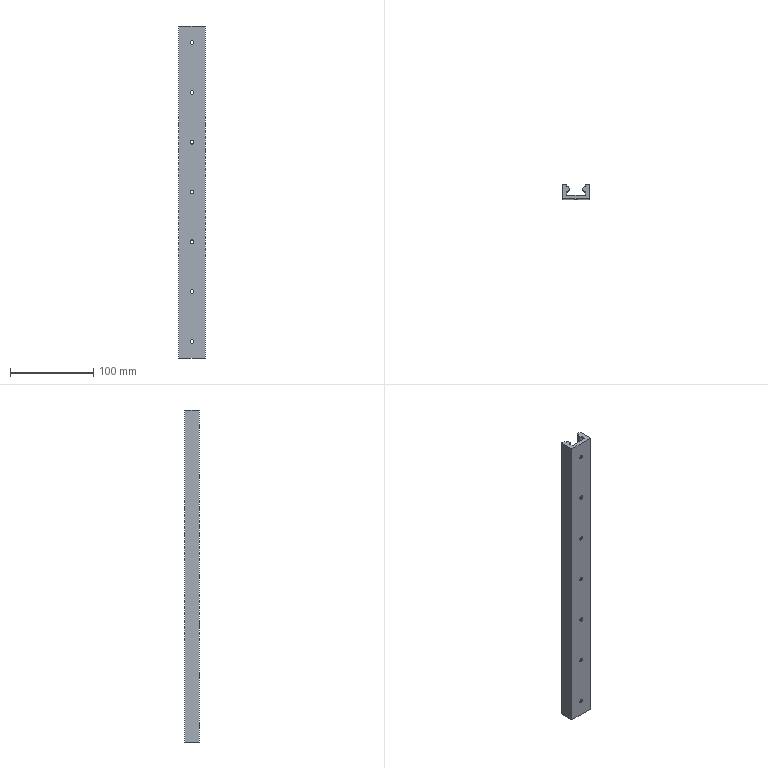Part | SolidWorks | features BaseBody 1 | 1 solid | 50 faces | box 32 x 17.5 x 400 mm | volume 119366 mm3 | cylinder 31 | plane 19 | commonest cylinder face diameters 4.5 x14 8 x14 6 x3
STEP:
#1=CARTESIAN_POINT('',(-16.,0.,400.));
#2=VERTEX_POINT('',#1);
#3=CARTESIAN_POINT('',(-10.95,0.,400.));
#4=VERTEX_POINT('',#3);
#5=CARTESIAN_POINT('',(-16.,0.,400.));
#6=DIRECTION('',(1.,0.,0.));
#7=VECTOR('',#6,1000.);
#8=LINE('',#5,#7);
#9=EDGE_CURVE('',#2,#4,#8,.T.);
#10=ORIENTED_EDGE('',*,*,#9,.F.);
#11=CARTESIAN_POINT('',(-16.,-17.5,400.));
#12=VERTEX_POINT('',#11);
#13=CARTESIAN_POINT('',(-16.,600.853,400.));
#14=DIRECTION('',(0.,-1.,0.));
#15=VECTOR('',#14,1000.);
#16=LINE('',#13,#15);
#17=EDGE_CURVE('',#2,#12,#16,.T.);
#18=ORIENTED_EDGE('',*,*,#17,.T.);
#19=CARTESIAN_POINT('',(16.,-17.5,400.));
#20=VERTEX_POINT('',#19);
#21=CARTESIAN_POINT('',(-16.,-17.5,400.));
#22=DIRECTION('',(1.,0.,0.));
#23=VECTOR('',#22,1000.);
#24=LINE('',#21,#23);
#25=EDGE_CURVE('',#12,#20,#24,.T.);
#26=ORIENTED_EDGE('',*,*,#25,.T.);
#27=CARTESIAN_POINT('',(16.,0.,400.));
#28=VERTEX_POINT('',#27);
#29=CARTESIAN_POINT('',(16.,600.853,400.));
#30=DIRECTION('',(0.,-1.,0.));
#31=VECTOR('',#30,1000.);
#32=LINE('',#29,#31);
#33=EDGE_CURVE('',#28,#20,#32,.T.);
#34=ORIENTED_EDGE('',*,*,#33,.F.);
#35=CARTESIAN_POINT('',(10.95,0.,400.));
#36=VERTEX_POINT('',#35);
#37=CARTESIAN_POINT('',(-16.,0.,400.));
#38=DIRECTION('',(1.,0.,0.));
#39=VECTOR('',#38,1000.);
#40=LINE('',#37,#39);
#41=EDGE_CURVE('',#36,#28,#40,.T.);
#42=ORIENTED_EDGE('',*,*,#41,.F.);
#43=CARTESIAN_POINT('',(10.95,-2.7,400.));
#44=VERTEX_POINT('',#43);
#45=CARTESIAN_POINT('',(10.95,0.,400.));
#46=DIRECTION('',(0.,1.,0.));
#47=VECTOR('',#46,1000.);
#48=LINE('',#45,#47);
#49=EDGE_CURVE('',#44,#36,#48,.T.);
#50=ORIENTED_EDGE('',*,*,#49,.F.);
#51=CARTESIAN_POINT('',(7.95,-5.7,400.));
#52=VERTEX_POINT('',#51);
#53=CARTESIAN_POINT('',(10.95,-5.7,400.));
#54=DIRECTION('',(0.,0.,1.));
#55=DIRECTION('',(-1.,0.,0.));
#56=AXIS2_PLACEMENT_3D('',#53,#54,#55);
#57=CIRCLE('',#56,3.);
#58=EDGE_CURVE('',#44,#52,#57,.T.);
#59=ORIENTED_EDGE('',*,*,#58,.T.);
#60=CARTESIAN_POINT('',(10.95,-8.7,400.));
#61=VERTEX_POINT('',#60);
#62=CARTESIAN_POINT('',(10.95,-5.7,400.));
#63=DIRECTION('',(0.,0.,1.));
#64=DIRECTION('',(-1.,0.,0.));
#65=AXIS2_PLACEMENT_3D('',#62,#63,#64);
#66=CIRCLE('',#65,3.);
#67=EDGE_CURVE('',#52,#61,#66,.T.);
#68=ORIENTED_EDGE('',*,*,#67,.T.);
#69=CARTESIAN_POINT('',(10.95,-13.1,400.));
#70=VERTEX_POINT('',#69);
#71=CARTESIAN_POINT('',(10.95,-8.7,400.));
#72=DIRECTION('',(0.,1.,0.));
#73=VECTOR('',#72,1000.);
#74=LINE('',#71,#73);
#75=EDGE_CURVE('',#70,#61,#74,.T.);
#76=ORIENTED_EDGE('',*,*,#75,.F.);
#77=CARTESIAN_POINT('',(-10.95,-13.1,400.));
#78=VERTEX_POINT('',#77);
#79=CARTESIAN_POINT('',(10.95,-13.1,400.));
#80=DIRECTION('',(1.,0.,0.));
#81=VECTOR('',#80,1000.);
#82=LINE('',#79,#81);
#83=EDGE_CURVE('',#78,#70,#82,.T.);
#84=ORIENTED_EDGE('',*,*,#83,.F.);
#85=CARTESIAN_POINT('',(-10.95,-8.7,400.));
#86=VERTEX_POINT('',#85);
#87=CARTESIAN_POINT('',(-10.95,-13.1,400.));
#88=DIRECTION('',(0.,-1.,0.));
#89=VECTOR('',#88,1000.);
#90=LINE('',#87,#89);
#91=EDGE_CURVE('',#86,#78,#90,.T.);
#92=ORIENTED_EDGE('',*,*,#91,.F.);
#93=CARTESIAN_POINT('',(-10.95,-2.7,400.));
#94=VERTEX_POINT('',#93);
#95=CARTESIAN_POINT('',(-10.95,-5.7,400.));
#96=DIRECTION('',(0.,0.,1.));
#97=DIRECTION('',(-1.,0.,0.));
#98=AXIS2_PLACEMENT_3D('',#95,#96,#97);
#99=CIRCLE('',#98,3.);
#100=EDGE_CURVE('',#86,#94,#99,.T.);
#101=ORIENTED_EDGE('',*,*,#100,.T.);
#102=CARTESIAN_POINT('',(-10.95,-2.7,400.));
#103=DIRECTION('',(0.,-1.,0.));
#104=VECTOR('',#103,1000.);
#105=LINE('',#102,#104);
#106=EDGE_CURVE('',#4,#94,#105,.T.);
#107=ORIENTED_EDGE('',*,*,#106,.F.);
#108=EDGE_LOOP('',(#10,#18,#26,#34,#42,#50,#59,#68,#76,#84,#92,#101,#107));
#109=FACE_OUTER_BOUND('',#108,.T.);
#110=CARTESIAN_POINT('',(-16.,600.853,400.));
#111=DIRECTION('',(0.,0.,-1.));
#112=DIRECTION('',(0.,-1.,0.));
#113=AXIS2_PLACEMENT_3D('',#110,#111,#112);
#114=PLANE('',#113);
#115=ADVANCED_FACE('',(#109),#114,.F.);
#116=CARTESIAN_POINT('',(0.,-16.,76.));
#117=VERTEX_POINT('',#116);
#118=CARTESIAN_POINT('',(0.,-16.,84.));
#119=VERTEX_POINT('',#118);
#120=CARTESIAN_POINT('',(0.,-16.,80.));
#121=DIRECTION('',(0.,1.,0.));
#122=DIRECTION('',(0.,0.,1.));
#123=AXIS2_PLACEMENT_3D('',#120,#121,#122);
#124=CIRCLE('',#123,4.);
#125=EDGE_CURVE('',#117,#119,#124,.T.);
#126=ORIENTED_EDGE('',*,*,#125,.F.);
#127=CARTESIAN_POINT('',(0.,-13.1,76.));
#128=VERTEX_POINT('',#127);
#129=CARTESIAN_POINT('',(0.,-13.1,76.));
#130=DIRECTION('',(0.,1.,0.));
#131=VECTOR('',#130,1000.);
#132=LINE('',#129,#131);
#133=EDGE_CURVE('',#117,#128,#132,.T.);
#134=ORIENTED_EDGE('',*,*,#133,.T.);
#135=CARTESIAN_POINT('',(0.,-13.1,84.));
#136=VERTEX_POINT('',#135);
#137=CARTESIAN_POINT('',(0.,-13.1,80.));
#138=DIRECTION('',(0.,1.,0.));
#139=DIRECTION('',(0.,0.,1.));
#140=AXIS2_PLACEMENT_3D('',#137,#138,#139);
#141=CIRCLE('',#140,4.);
#142=EDGE_CURVE('',#128,#136,#141,.T.);
#143=ORIENTED_EDGE('',*,*,#142,.T.);
#144=CARTESIAN_POINT('',(0.,-13.1,84.));
#145=DIRECTION('',(0.,1.,0.));
#146=VECTOR('',#145,1000.);
#147=LINE('',#144,#146);
#148=EDGE_CURVE('',#119,#136,#147,.T.);
#149=ORIENTED_EDGE('',*,*,#148,.F.);
#150=EDGE_LOOP('',(#126,#134,#143,#149));
#151=FACE_OUTER_BOUND('',#150,.T.);
#152=CARTESIAN_POINT('',(0.,-13.1,80.));
#153=DIRECTION('',(0.,1.,0.));
#154=DIRECTION('',(0.,0.,1.));
#155=AXIS2_PLACEMENT_3D('',#152,#153,#154);
#156=CYLINDRICAL_SURFACE('',#155,4.);
#157=ADVANCED_FACE('',(#151),#156,.F.);
#158=CARTESIAN_POINT('',(0.,-17.5,77.75));
#159=VERTEX_POINT('',#158);
#160=CARTESIAN_POINT('',(0.,-17.5,82.25));
#161=VERTEX_POINT('',#160);
#162=CARTESIAN_POINT('',(0.,-17.5,80.));
#163=DIRECTION('',(0.,1.,0.));
#164=DIRECTION('',(0.,0.,1.));
#165=AXIS2_PLACEMENT_3D('',#162,#163,#164);
#166=CIRCLE('',#165,2.25);
#167=EDGE_CURVE('',#159,#161,#166,.T.);
#168=ORIENTED_EDGE('',*,*,#167,.F.);
#169=CARTESIAN_POINT('',(0.,-16.,77.75));
#170=VERTEX_POINT('',#169);
#171=CARTESIAN_POINT('',(0.,-13.1,77.75));
#172=DIRECTION('',(0.,1.,0.));
#173=VECTOR('',#172,1000.);
#174=LINE('',#171,#173);
#175=EDGE_CURVE('',#159,#170,#174,.T.);
#176=ORIENTED_EDGE('',*,*,#175,.T.);
#177=CARTESIAN_POINT('',(0.,-16.,82.25));
#178=VERTEX_POINT('',#177);
#179=CARTESIAN_POINT('',(0.,-16.,80.));
#180=DIRECTION('',(0.,1.,0.));
#181=DIRECTION('',(0.,0.,1.));
#182=AXIS2_PLACEMENT_3D('',#179,#180,#181);
#183=CIRCLE('',#182,2.25);
#184=EDGE_CURVE('',#170,#178,#183,.T.);
#185=ORIENTED_EDGE('',*,*,#184,.T.);
#186=CARTESIAN_POINT('',(0.,-13.1,82.25));
#187=DIRECTION('',(0.,1.,0.));
#188=VECTOR('',#187,1000.);
#189=LINE('',#186,#188);
#190=EDGE_CURVE('',#161,#178,#189,.T.);
#191=ORIENTED_EDGE('',*,*,#190,.F.);
#192=EDGE_LOOP('',(#168,#176,#185,#191));
#193=FACE_OUTER_BOUND('',#192,.T.);
#194=CARTESIAN_POINT('',(0.,-13.1,80.));
#195=DIRECTION('',(0.,1.,0.));
#196=DIRECTION('',(0.,0.,1.));
#197=AXIS2_PLACEMENT_3D('',#194,#195,#196);
#198=CYLINDRICAL_SURFACE('',#197,2.25);
#199=ADVANCED_FACE('',(#193),#198,.F.);
#200=CARTESIAN_POINT('',(0.,-16.,16.));
#201=VERTEX_POINT('',#200);
#202=CARTESIAN_POINT('',(0.,-16.,24.));
#203=VERTEX_POINT('',#202);
#204=CARTESIAN_POINT('',(0.,-16.,20.));
#205=DIRECTION('',(0.,1.,0.));
#206=DIRECTION('',(0.,0.,1.));
#207=AXIS2_PLACEMENT_3D('',#204,#205,#206);
#208=CIRCLE('',#207,4.);
#209=EDGE_CURVE('',#201,#203,#208,.T.);
#210=ORIENTED_EDGE('',*,*,#209,.F.);
#211=CARTESIAN_POINT('',(0.,-13.1,16.));
#212=VERTEX_POINT('',#211);
#213=CARTESIAN_POINT('',(0.,-13.1,16.));
#214=DIRECTION('',(0.,1.,0.));
#215=VECTOR('',#214,1000.);
#216=LINE('',#213,#215);
#217=EDGE_CURVE('',#201,#212,#216,.T.);
#218=ORIENTED_EDGE('',*,*,#217,.T.);
#219=CARTESIAN_POINT('',(0.,-13.1,24.));
#220=VERTEX_POINT('',#219);
#221=CARTESIAN_POINT('',(0.,-13.1,20.));
#222=DIRECTION('',(0.,1.,0.));
#223=DIRECTION('',(0.,0.,1.));
#224=AXIS2_PLACEMENT_3D('',#221,#222,#223);
#225=CIRCLE('',#224,4.);
#226=EDGE_CURVE('',#212,#220,#225,.T.);
#227=ORIENTED_EDGE('',*,*,#226,.T.);
#228=CARTESIAN_POINT('',(0.,-13.1,24.));
#229=DIRECTION('',(0.,1.,0.));
#230=VECTOR('',#229,1000.);
#231=LINE('',#228,#230);
#232=EDGE_CURVE('',#203,#220,#231,.T.);
#233=ORIENTED_EDGE('',*,*,#232,.F.);
#234=EDGE_LOOP('',(#210,#218,#227,#233));
#235=FACE_OUTER_BOUND('',#234,.T.);
#236=CARTESIAN_POINT('',(0.,-13.1,20.));
#237=DIRECTION('',(0.,1.,0.));
#238=DIRECTION('',(0.,0.,1.));
#239=AXIS2_PLACEMENT_3D('',#236,#237,#238);
#240=CYLINDRICAL_SURFACE('',#239,4.);
#241=ADVANCED_FACE('',(#235),#240,.F.);
#242=CARTESIAN_POINT('',(0.,-17.5,17.75));
#243=VERTEX_POINT('',#242);
#244=CARTESIAN_POINT('',(0.,-17.5,22.25));
#245=VERTEX_POINT('',#244);
#246=CARTESIAN_POINT('',(0.,-17.5,20.));
#247=DIRECTION('',(0.,1.,0.));
#248=DIRECTION('',(0.,0.,1.));
#249=AXIS2_PLACEMENT_3D('',#246,#247,#248);
#250=CIRCLE('',#249,2.25);
#251=EDGE_CURVE('',#243,#245,#250,.T.);
#252=ORIENTED_EDGE('',*,*,#251,.F.);
#253=CARTESIAN_POINT('',(0.,-16.,17.75));
#254=VERTEX_POINT('',#253);
#255=CARTESIAN_POINT('',(0.,-13.1,17.75));
#256=DIRECTION('',(0.,1.,0.));
#257=VECTOR('',#256,1000.);
#258=LINE('',#255,#257);
#259=EDGE_CURVE('',#243,#254,#258,.T.);
#260=ORIENTED_EDGE('',*,*,#259,.T.);
#261=CARTESIAN_POINT('',(0.,-16.,22.25));
#262=VERTEX_POINT('',#261);
#263=CARTESIAN_POINT('',(0.,-16.,20.));
#264=DIRECTION('',(0.,1.,0.));
#265=DIRECTION('',(0.,0.,1.));
#266=AXIS2_PLACEMENT_3D('',#263,#264,#265);
#267=CIRCLE('',#266,2.25);
#268=EDGE_CURVE('',#254,#262,#267,.T.);
#269=ORIENTED_EDGE('',*,*,#268,.T.);
#270=CARTESIAN_POINT('',(0.,-13.1,22.25));
#271=DIRECTION('',(0.,1.,0.));
#272=VECTOR('',#271,1000.);
#273=LINE('',#270,#272);
#274=EDGE_CURVE('',#245,#262,#273,.T.);
#275=ORIENTED_EDGE('',*,*,#274,.F.);
#276=EDGE_LOOP('',(#252,#260,#269,#275));
#277=FACE_OUTER_BOUND('',#276,.T.);
#278=CARTESIAN_POINT('',(0.,-13.1,20.));
#279=DIRECTION('',(0.,1.,0.));
#280=DIRECTION('',(0.,0.,1.));
#281=AXIS2_PLACEMENT_3D('',#278,#279,#280);
#282=CYLINDRICAL_SURFACE('',#281,2.25);
#283=ADVANCED_FACE('',(#277),#282,.F.);
#284=CARTESIAN_POINT('',(0.,-16.,136.));
#285=VERTEX_POINT('',#284);
#286=CARTESIAN_POINT('',(0.,-16.,144.));
#287=VERTEX_POINT('',#286);
#288=CARTESIAN_POINT('',(0.,-16.,140.));
#289=DIRECTION('',(0.,1.,0.));
#290=DIRECTION('',(0.,0.,1.));
#291=AXIS2_PLACEMENT_3D('',#288,#289,#290);
#292=CIRCLE('',#291,4.);
#293=EDGE_CURVE('',#285,#287,#292,.T.);
#294=ORIENTED_EDGE('',*,*,#293,.F.);
#295=CARTESIAN_POINT('',(0.,-13.1,136.));
#296=VERTEX_POINT('',#295);
#297=CARTESIAN_POINT('',(0.,-13.1,136.));
#298=DIRECTION('',(0.,1.,0.));
#299=VECTOR('',#298,1000.);
#300=LINE('',#297,#299);
#301=EDGE_CURVE('',#285,#296,#300,.T.);
#302=ORIENTED_EDGE('',*,*,#301,.T.);
#303=CARTESIAN_POINT('',(0.,-13.1,144.));
#304=VERTEX_POINT('',#303);
#305=CARTESIAN_POINT('',(0.,-13.1,140.));
#306=DIRECTION('',(0.,1.,0.));
#307=DIRECTION('',(0.,0.,1.));
#308=AXIS2_PLACEMENT_3D('',#305,#306,#307);
#309=CIRCLE('',#308,4.);
#310=EDGE_CURVE('',#296,#304,#309,.T.);
#311=ORIENTED_EDGE('',*,*,#310,.T.);
#312=CARTESIAN_POINT('',(0.,-13.1,144.));
#313=DIRECTION('',(0.,1.,0.));
#314=VECTOR('',#313,1000.);
#315=LINE('',#312,#314);
#316=EDGE_CURVE('',#287,#304,#315,.T.);
#317=ORIENTED_EDGE('',*,*,#316,.F.);
#318=EDGE_LOOP('',(#294,#302,#311,#317));
#319=FACE_OUTER_BOUND('',#318,.T.);
#320=CARTESIAN_POINT('',(0.,-13.1,140.));
#321=DIRECTION('',(0.,1.,0.));
#322=DIRECTION('',(0.,0.,1.));
#323=AXIS2_PLACEMENT_3D('',#320,#321,#322);
#324=CYLINDRICAL_SURFACE('',#323,4.);
#325=ADVANCED_FACE('',(#319),#324,.F.);
#326=CARTESIAN_POINT('',(0.,-17.5,137.75));
#327=VERTEX_POINT('',#326);
#328=CARTESIAN_POINT('',(0.,-17.5,142.25));
#329=VERTEX_POINT('',#328);
#330=CARTESIAN_POINT('',(0.,-17.5,140.));
#331=DIRECTION('',(0.,1.,0.));
#332=DIRECTION('',(0.,0.,1.));
#333=AXIS2_PLACEMENT_3D('',#330,#331,#332);
#334=CIRCLE('',#333,2.25);
#335=EDGE_CURVE('',#327,#329,#334,.T.);
#336=ORIENTED_EDGE('',*,*,#335,.F.);
#337=CARTESIAN_POINT('',(0.,-16.,137.75));
#338=VERTEX_POINT('',#337);
#339=CARTESIAN_POINT('',(0.,-13.1,137.75));
#340=DIRECTION('',(0.,1.,0.));
#341=VECTOR('',#340,1000.);
#342=LINE('',#339,#341);
#343=EDGE_CURVE('',#327,#338,#342,.T.);
#344=ORIENTED_EDGE('',*,*,#343,.T.);
#345=CARTESIAN_POINT('',(0.,-16.,142.25));
#346=VERTEX_POINT('',#345);
#347=CARTESIAN_POINT('',(0.,-16.,140.));
#348=DIRECTION('',(0.,1.,0.));
#349=DIRECTION('',(0.,0.,1.));
#350=AXIS2_PLACEMENT_3D('',#347,#348,#349);
#351=CIRCLE('',#350,2.25);
#352=EDGE_CURVE('',#338,#346,#351,.T.);
#353=ORIENTED_EDGE('',*,*,#352,.T.);
#354=CARTESIAN_POINT('',(0.,-13.1,142.25));
#355=DIRECTION('',(0.,1.,0.));
#356=VECTOR('',#355,1000.);
#357=LINE('',#354,#356);
#358=EDGE_CURVE('',#329,#346,#357,.T.);
#359=ORIENTED_EDGE('',*,*,#358,.F.);
#360=EDGE_LOOP('',(#336,#344,#353,#359));
#361=FACE_OUTER_BOUND('',#360,.T.);
#362=CARTESIAN_POINT('',(0.,-13.1,140.));
#363=DIRECTION('',(0.,1.,0.));
#364=DIRECTION('',(0.,0.,1.));
#365=AXIS2_PLACEMENT_3D('',#362,#363,#364);
#366=CYLINDRICAL_SURFACE('',#365,2.25);
#367=ADVANCED_FACE('',(#361),#366,.F.);
#368=CARTESIAN_POINT('',(0.,-16.,196.));
#369=VERTEX_POINT('',#368);
#370=CARTESIAN_POINT('',(0.,-16.,204.));
#371=VERTEX_POINT('',#370);
#372=CARTESIAN_POINT('',(0.,-16.,200.));
#373=DIRECTION('',(0.,1.,0.));
#374=DIRECTION('',(0.,0.,1.));
#375=AXIS2_PLACEMENT_3D('',#372,#373,#374);
#376=CIRCLE('',#375,4.);
#377=EDGE_CURVE('',#369,#371,#376,.T.);
#378=ORIENTED_EDGE('',*,*,#377,.F.);
#379=CARTESIAN_POINT('',(0.,-13.1,196.));
#380=VERTEX_POINT('',#379);
#381=CARTESIAN_POINT('',(0.,-13.1,196.));
#382=DIRECTION('',(0.,1.,0.));
#383=VECTOR('',#382,1000.);
#384=LINE('',#381,#383);
#385=EDGE_CURVE('',#369,#380,#384,.T.);
#386=ORIENTED_EDGE('',*,*,#385,.T.);
#387=CARTESIAN_POINT('',(0.,-13.1,204.));
#388=VERTEX_POINT('',#387);
#389=CARTESIAN_POINT('',(0.,-13.1,200.));
#390=DIRECTION('',(0.,1.,0.));
#391=DIRECTION('',(0.,0.,1.));
#392=AXIS2_PLACEMENT_3D('',#389,#390,#391);
#393=CIRCLE('',#392,4.);
#394=EDGE_CURVE('',#380,#388,#393,.T.);
#395=ORIENTED_EDGE('',*,*,#394,.T.);
#396=CARTESIAN_POINT('',(0.,-13.1,204.));
#397=DIRECTION('',(0.,1.,0.));
#398=VECTOR('',#397,1000.);
#399=LINE('',#396,#398);
#400=EDGE_CURVE('',#371,#388,#399,.T.);
#401=ORIENTED_EDGE('',*,*,#400,.F.);
#402=EDGE_LOOP('',(#378,#386,#395,#401));
#403=FACE_OUTER_BOUND('',#402,.T.);
#404=CARTESIAN_POINT('',(0.,-13.1,200.));
#405=DIRECTION('',(0.,1.,0.));
#406=DIRECTION('',(0.,0.,1.));
#407=AXIS2_PLACEMENT_3D('',#404,#405,#406);
#408=CYLINDRICAL_SURFACE('',#407,4.);
#409=ADVANCED_FACE('',(#403),#408,.F.);
#410=CARTESIAN_POINT('',(0.,-17.5,197.75));
#411=VERTEX_POINT('',#410);
#412=CARTESIAN_POINT('',(0.,-17.5,202.25));
#413=VERTEX_POINT('',#412);
#414=CARTESIAN_POINT('',(0.,-17.5,200.));
#415=DIRECTION('',(0.,1.,0.));
#416=DIRECTION('',(0.,0.,1.));
#417=AXIS2_PLACEMENT_3D('',#414,#415,#416);
#418=CIRCLE('',#417,2.25);
#419=EDGE_CURVE('',#411,#413,#418,.T.);
#420=ORIENTED_EDGE('',*,*,#419,.F.);
#421=CARTESIAN_POINT('',(0.,-16.,197.75));
#422=VERTEX_POINT('',#421);
#423=CARTESIAN_POINT('',(0.,-13.1,197.75));
#424=DIRECTION('',(0.,1.,0.));
#425=VECTOR('',#424,1000.);
#426=LINE('',#423,#425);
#427=EDGE_CURVE('',#411,#422,#426,.T.);
#428=ORIENTED_EDGE('',*,*,#427,.T.);
#429=CARTESIAN_POINT('',(0.,-16.,202.25));
#430=VERTEX_POINT('',#429);
#431=CARTESIAN_POINT('',(0.,-16.,200.));
#432=DIRECTION('',(0.,1.,0.));
#433=DIRECTION('',(0.,0.,1.));
#434=AXIS2_PLACEMENT_3D('',#431,#432,#433);
#435=CIRCLE('',#434,2.25);
#436=EDGE_CURVE('',#422,#430,#435,.T.);
#437=ORIENTED_EDGE('',*,*,#436,.T.);
#438=CARTESIAN_POINT('',(0.,-13.1,202.25));
#439=DIRECTION('',(0.,1.,0.));
#440=VECTOR('',#439,1000.);
#441=LINE('',#438,#440);
#442=EDGE_CURVE('',#413,#430,#441,.T.);
#443=ORIENTED_EDGE('',*,*,#442,.F.);
#444=EDGE_LOOP('',(#420,#428,#437,#443));
#445=FACE_OUTER_BOUND('',#444,.T.);
#446=CARTESIAN_POINT('',(0.,-13.1,200.));
#447=DIRECTION('',(0.,1.,0.));
#448=DIRECTION('',(0.,0.,1.));
#449=AXIS2_PLACEMENT_3D('',#446,#447,#448);
#450=CYLINDRICAL_SURFACE('',#449,2.25);
#451=ADVANCED_FACE('',(#445),#450,.F.);
#452=CARTESIAN_POINT('',(0.,-16.,256.));
#453=VERTEX_POINT('',#452);
#454=CARTESIAN_POINT('',(0.,-16.,264.));
#455=VERTEX_POINT('',#454);
#456=CARTESIAN_POINT('',(0.,-16.,260.));
#457=DIRECTION('',(0.,1.,0.));
#458=DIRECTION('',(0.,0.,1.));
#459=AXIS2_PLACEMENT_3D('',#456,#457,#458);
#460=CIRCLE('',#459,4.);
#461=EDGE_CURVE('',#453,#455,#460,.T.);
#462=ORIENTED_EDGE('',*,*,#461,.F.);
#463=CARTESIAN_POINT('',(0.,-13.1,256.));
#464=VERTEX_POINT('',#463);
#465=CARTESIAN_POINT('',(0.,-13.1,256.));
#466=DIRECTION('',(0.,1.,0.));
#467=VECTOR('',#466,1000.);
#468=LINE('',#465,#467);
#469=EDGE_CURVE('',#453,#464,#468,.T.);
#470=ORIENTED_EDGE('',*,*,#469,.T.);
#471=CARTESIAN_POINT('',(0.,-13.1,264.));
#472=VERTEX_POINT('',#471);
#473=CARTESIAN_POINT('',(0.,-13.1,260.));
#474=DIRECTION('',(0.,1.,0.));
#475=DIRECTION('',(0.,0.,1.));
#476=AXIS2_PLACEMENT_3D('',#473,#474,#475);
#477=CIRCLE('',#476,4.);
#478=EDGE_CURVE('',#464,#472,#477,.T.);
#479=ORIENTED_EDGE('',*,*,#478,.T.);
#480=CARTESIAN_POINT('',(0.,-13.1,264.));
#481=DIRECTION('',(0.,1.,0.));
#482=VECTOR('',#481,1000.);
#483=LINE('',#480,#482);
#484=EDGE_CURVE('',#455,#472,#483,.T.);
#485=ORIENTED_EDGE('',*,*,#484,.F.);
#486=EDGE_LOOP('',(#462,#470,#479,#485));
#487=FACE_OUTER_BOUND('',#486,.T.);
#488=CARTESIAN_POINT('',(0.,-13.1,260.));
#489=DIRECTION('',(0.,1.,0.));
#490=DIRECTION('',(0.,0.,1.));
#491=AXIS2_PLACEMENT_3D('',#488,#489,#490);
#492=CYLINDRICAL_SURFACE('',#491,4.);
#493=ADVANCED_FACE('',(#487),#492,.F.);
#494=CARTESIAN_POINT('',(0.,-17.5,257.75));
#495=VERTEX_POINT('',#494);
#496=CARTESIAN_POINT('',(0.,-17.5,262.25));
#497=VERTEX_POINT('',#496);
#498=CARTESIAN_POINT('',(0.,-17.5,260.));
#499=DIRECTION('',(0.,1.,0.));
#500=DIRECTION('',(0.,0.,1.));
#501=AXIS2_PLACEMENT_3D('',#498,#499,#500);
#502=CIRCLE('',#501,2.25);
#503=EDGE_CURVE('',#495,#497,#502,.T.);
#504=ORIENTED_EDGE('',*,*,#503,.F.);
#505=CARTESIAN_POINT('',(0.,-16.,257.75));
#506=VERTEX_POINT('',#505);
#507=CARTESIAN_POINT('',(0.,-13.1,257.75));
#508=DIRECTION('',(0.,1.,0.));
#509=VECTOR('',#508,1000.);
#510=LINE('',#507,#509);
#511=EDGE_CURVE('',#495,#506,#510,.T.);
#512=ORIENTED_EDGE('',*,*,#511,.T.);
#513=CARTESIAN_POINT('',(0.,-16.,262.25));
#514=VERTEX_POINT('',#513);
#515=CARTESIAN_POINT('',(0.,-16.,260.));
#516=DIRECTION('',(0.,1.,0.));
#517=DIRECTION('',(0.,0.,1.));
#518=AXIS2_PLACEMENT_3D('',#515,#516,#517);
#519=CIRCLE('',#518,2.25);
#520=EDGE_CURVE('',#506,#514,#519,.T.);
#521=ORIENTED_EDGE('',*,*,#520,.T.);
#522=CARTESIAN_POINT('',(0.,-13.1,262.25));
#523=DIRECTION('',(0.,1.,0.));
#524=VECTOR('',#523,1000.);
#525=LINE('',#522,#524);
#526=EDGE_CURVE('',#497,#514,#525,.T.);
#527=ORIENTED_EDGE('',*,*,#526,.F.);
#528=EDGE_LOOP('',(#504,#512,#521,#527));
#529=FACE_OUTER_BOUND('',#528,.T.);
#530=CARTESIAN_POINT('',(0.,-13.1,260.));
#531=DIRECTION('',(0.,1.,0.));
#532=DIRECTION('',(0.,0.,1.));
#533=AXIS2_PLACEMENT_3D('',#530,#531,#532);
#534=CYLINDRICAL_SURFACE('',#533,2.25);
#535=ADVANCED_FACE('',(#529),#534,.F.);
#536=CARTESIAN_POINT('',(0.,-16.,316.));
#537=VERTEX_POINT('',#536);
#538=CARTESIAN_POINT('',(0.,-16.,324.));
#539=VERTEX_POINT('',#538);
#540=CARTESIAN_POINT('',(0.,-16.,320.));
#541=DIRECTION('',(0.,1.,0.));
#542=DIRECTION('',(0.,0.,1.));
#543=AXIS2_PLACEMENT_3D('',#540,#541,#542);
#544=CIRCLE('',#543,4.);
#545=EDGE_CURVE('',#537,#539,#544,.T.);
#546=ORIENTED_EDGE('',*,*,#545,.F.);
#547=CARTESIAN_POINT('',(0.,-13.1,316.));
#548=VERTEX_POINT('',#547);
#549=CARTESIAN_POINT('',(0.,-13.1,316.));
#550=DIRECTION('',(0.,1.,0.));
#551=VECTOR('',#550,1000.);
#552=LINE('',#549,#551);
#553=EDGE_CURVE('',#537,#548,#552,.T.);
#554=ORIENTED_EDGE('',*,*,#553,.T.);
#555=CARTESIAN_POINT('',(0.,-13.1,324.));
#556=VERTEX_POINT('',#555);
#557=CARTESIAN_POINT('',(0.,-13.1,320.));
#558=DIRECTION('',(0.,1.,0.));
#559=DIRECTION('',(0.,0.,1.));
#560=AXIS2_PLACEMENT_3D('',#557,#558,#559);
#561=CIRCLE('',#560,4.);
#562=EDGE_CURVE('',#548,#556,#561,.T.);
#563=ORIENTED_EDGE('',*,*,#562,.T.);
#564=CARTESIAN_POINT('',(0.,-13.1,324.));
#565=DIRECTION('',(0.,1.,0.));
#566=VECTOR('',#565,1000.);
#567=LINE('',#564,#566);
#568=EDGE_CURVE('',#539,#556,#567,.T.);
#569=ORIENTED_EDGE('',*,*,#568,.F.);
#570=EDGE_LOOP('',(#546,#554,#563,#569));
#571=FACE_OUTER_BOUND('',#570,.T.);
#572=CARTESIAN_POINT('',(0.,-13.1,320.));
#573=DIRECTION('',(0.,1.,0.));
#574=DIRECTION('',(0.,0.,1.));
#575=AXIS2_PLACEMENT_3D('',#572,#573,#574);
#576=CYLINDRICAL_SURFACE('',#575,4.);
#577=ADVANCED_FACE('',(#571),#576,.F.);
#578=CARTESIAN_POINT('',(0.,-17.5,317.75));
#579=VERTEX_POINT('',#578);
#580=CARTESIAN_POINT('',(0.,-17.5,322.25));
#581=VERTEX_POINT('',#580);
#582=CARTESIAN_POINT('',(0.,-17.5,320.));
#583=DIRECTION('',(0.,1.,0.));
#584=DIRECTION('',(0.,0.,1.));
#585=AXIS2_PLACEMENT_3D('',#582,#583,#584);
#586=CIRCLE('',#585,2.25);
#587=EDGE_CURVE('',#579,#581,#586,.T.);
#588=ORIENTED_EDGE('',*,*,#587,.F.);
#589=CARTESIAN_POINT('',(0.,-16.,317.75));
#590=VERTEX_POINT('',#589);
#591=CARTESIAN_POINT('',(0.,-13.1,317.75));
#592=DIRECTION('',(0.,1.,0.));
#593=VECTOR('',#592,1000.);
#594=LINE('',#591,#593);
#595=EDGE_CURVE('',#579,#590,#594,.T.);
#596=ORIENTED_EDGE('',*,*,#595,.T.);
#597=CARTESIAN_POINT('',(0.,-16.,322.25));
#598=VERTEX_POINT('',#597);
#599=CARTESIAN_POINT('',(0.,-16.,320.));
#600=DIRECTION('',(0.,1.,0.));
#601=DIRECTION('',(0.,0.,1.));
#602=AXIS2_PLACEMENT_3D('',#599,#600,#601);
#603=CIRCLE('',#602,2.25);
#604=EDGE_CURVE('',#590,#598,#603,.T.);
#605=ORIENTED_EDGE('',*,*,#604,.T.);
#606=CARTESIAN_POINT('',(0.,-13.1,322.25));
#607=DIRECTION('',(0.,1.,0.));
#608=VECTOR('',#607,1000.);
#609=LINE('',#606,#608);
#610=EDGE_CURVE('',#581,#598,#609,.T.);
#611=ORIENTED_EDGE('',*,*,#610,.F.);
#612=EDGE_LOOP('',(#588,#596,#605,#611));
#613=FACE_OUTER_BOUND('',#612,.T.);
#614=CARTESIAN_POINT('',(0.,-13.1,320.));
#615=DIRECTION('',(0.,1.,0.));
#616=DIRECTION('',(0.,0.,1.));
#617=AXIS2_PLACEMENT_3D('',#614,#615,#616);
#618=CYLINDRICAL_SURFACE('',#617,2.25);
#619=ADVANCED_FACE('',(#613),#618,.F.);
#620=CARTESIAN_POINT('',(0.,-16.,376.));
#621=VERTEX_POINT('',#620);
#622=CARTESIAN_POINT('',(0.,-16.,384.));
#623=VERTEX_POINT('',#622);
#624=CARTESIAN_POINT('',(0.,-16.,380.));
#625=DIRECTION('',(0.,1.,0.));
#626=DIRECTION('',(0.,0.,1.));
#627=AXIS2_PLACEMENT_3D('',#624,#625,#626);
#628=CIRCLE('',#627,4.);
#629=EDGE_CURVE('',#621,#623,#628,.T.);
#630=ORIENTED_EDGE('',*,*,#629,.F.);
#631=CARTESIAN_POINT('',(0.,-13.1,376.));
#632=VERTEX_POINT('',#631);
#633=CARTESIAN_POINT('',(0.,-13.1,376.));
#634=DIRECTION('',(0.,1.,0.));
#635=VECTOR('',#634,1000.);
#636=LINE('',#633,#635);
#637=EDGE_CURVE('',#621,#632,#636,.T.);
#638=ORIENTED_EDGE('',*,*,#637,.T.);
#639=CARTESIAN_POINT('',(0.,-13.1,384.));
#640=VERTEX_POINT('',#639);
#641=CARTESIAN_POINT('',(0.,-13.1,380.));
#642=DIRECTION('',(0.,1.,0.));
#643=DIRECTION('',(0.,0.,1.));
#644=AXIS2_PLACEMENT_3D('',#641,#642,#643);
#645=CIRCLE('',#644,4.);
#646=EDGE_CURVE('',#632,#640,#645,.T.);
#647=ORIENTED_EDGE('',*,*,#646,.T.);
#648=CARTESIAN_POINT('',(0.,-13.1,384.));
#649=DIRECTION('',(0.,1.,0.));
#650=VECTOR('',#649,1000.);
#651=LINE('',#648,#650);
#652=EDGE_CURVE('',#623,#640,#651,.T.);
#653=ORIENTED_EDGE('',*,*,#652,.F.);
#654=EDGE_LOOP('',(#630,#638,#647,#653));
#655=FACE_OUTER_BOUND('',#654,.T.);
#656=CARTESIAN_POINT('',(0.,-13.1,380.));
#657=DIRECTION('',(0.,1.,0.));
#658=DIRECTION('',(0.,0.,1.));
#659=AXIS2_PLACEMENT_3D('',#656,#657,#658);
#660=CYLINDRICAL_SURFACE('',#659,4.);
#661=ADVANCED_FACE('',(#655),#660,.F.);
#662=CARTESIAN_POINT('',(0.,-17.5,377.75));
#663=VERTEX_POINT('',#662);
#664=CARTESIAN_POINT('',(0.,-17.5,382.25));
#665=VERTEX_POINT('',#664);
#666=CARTESIAN_POINT('',(0.,-17.5,380.));
#667=DIRECTION('',(0.,1.,0.));
#668=DIRECTION('',(0.,0.,1.));
#669=AXIS2_PLACEMENT_3D('',#666,#667,#668);
#670=CIRCLE('',#669,2.25);
#671=EDGE_CURVE('',#663,#665,#670,.T.);
#672=ORIENTED_EDGE('',*,*,#671,.F.);
#673=CARTESIAN_POINT('',(0.,-16.,377.75));
#674=VERTEX_POINT('',#673);
#675=CARTESIAN_POINT('',(0.,-13.1,377.75));
#676=DIRECTION('',(0.,1.,0.));
#677=VECTOR('',#676,1000.);
#678=LINE('',#675,#677);
#679=EDGE_CURVE('',#663,#674,#678,.T.);
#680=ORIENTED_EDGE('',*,*,#679,.T.);
#681=CARTESIAN_POINT('',(0.,-16.,382.25));
#682=VERTEX_POINT('',#681);
#683=CARTESIAN_POINT('',(0.,-16.,380.));
#684=DIRECTION('',(0.,1.,0.));
#685=DIRECTION('',(0.,0.,1.));
#686=AXIS2_PLACEMENT_3D('',#683,#684,#685);
#687=CIRCLE('',#686,2.25);
#688=EDGE_CURVE('',#674,#682,#687,.T.);
#689=ORIENTED_EDGE('',*,*,#688,.T.);
#690=CARTESIAN_POINT('',(0.,-13.1,382.25));
#691=DIRECTION('',(0.,1.,0.));
#692=VECTOR('',#691,1000.);
#693=LINE('',#690,#692);
#694=EDGE_CURVE('',#665,#682,#693,.T.);
#695=ORIENTED_EDGE('',*,*,#694,.F.);
#696=EDGE_LOOP('',(#672,#680,#689,#695));
#697=FACE_OUTER_BOUND('',#696,.T.);
#698=CARTESIAN_POINT('',(0.,-13.1,380.));
#699=DIRECTION('',(0.,1.,0.));
#700=DIRECTION('',(0.,0.,1.));
#701=AXIS2_PLACEMENT_3D('',#698,#699,#700);
#702=CYLINDRICAL_SURFACE('',#701,2.25);
#703=ADVANCED_FACE('',(#697),#702,.F.);
#704=ORIENTED_EDGE('',*,*,#67,.F.);
#705=CARTESIAN_POINT('',(7.95,-5.7,0.));
#706=VERTEX_POINT('',#705);
#707=CARTESIAN_POINT('',(7.95,-5.7,1000.));
#708=DIRECTION('',(0.,0.,-1.));
#709=VECTOR('',#708,1000.);
#710=LINE('',#707,#709);
#711=EDGE_CURVE('',#52,#706,#710,.T.);
#712=ORIENTED_EDGE('',*,*,#711,.T.);
#713=CARTESIAN_POINT('',(10.95,-8.7,0.));
#714=VERTEX_POINT('',#713);
#715=CARTESIAN_POINT('',(10.95,-5.7,0.));
#716=DIRECTION('',(0.,0.,1.));
#717=DIRECTION('',(1.,0.,0.));
#718=AXIS2_PLACEMENT_3D('',#715,#716,#717);
#719=CIRCLE('',#718,3.);
#720=EDGE_CURVE('',#706,#714,#719,.T.);
#721=ORIENTED_EDGE('',*,*,#720,.T.);
#722=CARTESIAN_POINT('',(10.95,-8.7,1000.));
#723=DIRECTION('',(0.,0.,-1.));
#724=VECTOR('',#723,1000.);
#725=LINE('',#722,#724);
#726=EDGE_CURVE('',#61,#714,#725,.T.);
#727=ORIENTED_EDGE('',*,*,#726,.F.);
#728=EDGE_LOOP('',(#704,#712,#721,#727));
#729=FACE_OUTER_BOUND('',#728,.T.);
#730=CARTESIAN_POINT('',(10.95,-5.7,1000.));
#731=DIRECTION('',(0.,0.,-1.));
#732=DIRECTION('',(-1.,0.,0.));
#733=AXIS2_PLACEMENT_3D('',#730,#731,#732);
#734=CYLINDRICAL_SURFACE('',#733,3.);
#735=ADVANCED_FACE('',(#729),#734,.T.);
#736=ORIENTED_EDGE('',*,*,#9,.T.);
#737=CARTESIAN_POINT('',(-10.95,0.,0.));
#738=VERTEX_POINT('',#737);
#739=CARTESIAN_POINT('',(-10.95,0.,1000.));
#740=DIRECTION('',(0.,0.,-1.));
#741=VECTOR('',#740,1000.);
#742=LINE('',#739,#741);
#743=EDGE_CURVE('',#4,#738,#742,.T.);
#744=ORIENTED_EDGE('',*,*,#743,.T.);
#745=CARTESIAN_POINT('',(-16.,0.,0.));
#746=VERTEX_POINT('',#745);
#747=CARTESIAN_POINT('',(16.,0.,0.));
#748=DIRECTION('',(-1.,0.,0.));
#749=VECTOR('',#748,1000.);
#750=LINE('',#747,#749);
#751=EDGE_CURVE('',#738,#746,#750,.T.);
#752=ORIENTED_EDGE('',*,*,#751,.T.);
#753=CARTESIAN_POINT('',(-16.,0.,0.));
#754=DIRECTION('',(0.,0.,1.));
#755=VECTOR('',#754,1000.);
#756=LINE('',#753,#755);
#757=EDGE_CURVE('',#746,#2,#756,.T.);
#758=ORIENTED_EDGE('',*,*,#757,.T.);
#759=EDGE_LOOP('',(#736,#744,#752,#758));
#760=FACE_OUTER_BOUND('',#759,.T.);
#761=CARTESIAN_POINT('',(0.,0.,0.));
#762=DIRECTION('',(0.,1.,0.));
#763=DIRECTION('',(1.,0.,0.));
#764=AXIS2_PLACEMENT_3D('',#761,#762,#763);
#765=PLANE('',#764);
#766=ADVANCED_FACE('',(#760),#765,.T.);
#767=ORIENTED_EDGE('',*,*,#33,.T.);
#768=CARTESIAN_POINT('',(16.,-17.5,0.));
#769=VERTEX_POINT('',#768);
#770=CARTESIAN_POINT('',(16.,-17.5,1000.));
#771=DIRECTION('',(0.,0.,-1.));
#772=VECTOR('',#771,1000.);
#773=LINE('',#770,#772);
#774=EDGE_CURVE('',#20,#769,#773,.T.);
#775=ORIENTED_EDGE('',*,*,#774,.T.);
#776=CARTESIAN_POINT('',(16.,0.,0.));
#777=VERTEX_POINT('',#776);
#778=CARTESIAN_POINT('',(16.,-17.5,0.));
#779=DIRECTION('',(0.,1.,0.));
#780=VECTOR('',#779,1000.);
#781=LINE('',#778,#780);
#782=EDGE_CURVE('',#769,#777,#781,.T.);
#783=ORIENTED_EDGE('',*,*,#782,.T.);
#784=CARTESIAN_POINT('',(16.,0.,1000.));
#785=DIRECTION('',(0.,0.,-1.));
#786=VECTOR('',#785,1000.);
#787=LINE('',#784,#786);
#788=EDGE_CURVE('',#28,#777,#787,.T.);
#789=ORIENTED_EDGE('',*,*,#788,.F.);
#790=EDGE_LOOP('',(#767,#775,#783,#789));
#791=FACE_OUTER_BOUND('',#790,.T.);
#792=CARTESIAN_POINT('',(16.,-17.5,1000.));
#793=DIRECTION('',(1.,0.,0.));
#794=DIRECTION('',(0.,1.,0.));
#795=AXIS2_PLACEMENT_3D('',#792,#793,#794);
#796=PLANE('',#795);
#797=ADVANCED_FACE('',(#791),#796,.T.);
#798=ORIENTED_EDGE('',*,*,#17,.F.);
#799=ORIENTED_EDGE('',*,*,#757,.F.);
#800=CARTESIAN_POINT('',(-16.,-17.5,0.));
#801=VERTEX_POINT('',#800);
#802=CARTESIAN_POINT('',(-16.,-17.5,0.));
#803=DIRECTION('',(0.,1.,0.));
#804=VECTOR('',#803,1000.);
#805=LINE('',#802,#804);
#806=EDGE_CURVE('',#801,#746,#805,.T.);
#807=ORIENTED_EDGE('',*,*,#806,.F.);
#808=CARTESIAN_POINT('',(-16.,-17.5,0.));
#809=DIRECTION('',(0.,0.,1.));
#810=VECTOR('',#809,1000.);
#811=LINE('',#808,#810);
#812=EDGE_CURVE('',#801,#12,#811,.T.);
#813=ORIENTED_EDGE('',*,*,#812,.T.);
#814=EDGE_LOOP('',(#798,#799,#807,#813));
#815=FACE_OUTER_BOUND('',#814,.T.);
#816=CARTESIAN_POINT('',(-16.,-17.5,0.));
#817=DIRECTION('',(-1.,0.,0.));
#818=DIRECTION('',(0.,0.,1.));
#819=AXIS2_PLACEMENT_3D('',#816,#817,#818);
#820=PLANE('',#819);
#821=ADVANCED_FACE('',(#815),#820,.T.);
#822=CARTESIAN_POINT('',(-10.95,-2.7,0.));
#823=VERTEX_POINT('',#822);
#824=CARTESIAN_POINT('',(-10.95,-2.7,0.));
#825=DIRECTION('',(0.,1.,0.));
#826=VECTOR('',#825,1000.);
#827=LINE('',#824,#826);
#828=EDGE_CURVE('',#823,#738,#827,.T.);
#829=ORIENTED_EDGE('',*,*,#828,.F.);
#830=CARTESIAN_POINT('',(-10.95,-8.7,0.));
#831=VERTEX_POINT('',#830);
#832=CARTESIAN_POINT('',(-10.95,-5.7,0.));
#833=DIRECTION('',(0.,0.,1.));
#834=DIRECTION('',(1.,0.,0.));
#835=AXIS2_PLACEMENT_3D('',#832,#833,#834);
#836=CIRCLE('',#835,3.);
#837=EDGE_CURVE('',#831,#823,#836,.T.);
#838=ORIENTED_EDGE('',*,*,#837,.F.);
#839=CARTESIAN_POINT('',(-10.95,-13.1,0.));
#840=VERTEX_POINT('',#839);
#841=CARTESIAN_POINT('',(-10.95,-13.1,0.));
#842=DIRECTION('',(0.,1.,0.));
#843=VECTOR('',#842,1000.);
#844=LINE('',#841,#843);
#845=EDGE_CURVE('',#840,#831,#844,.T.);
#846=ORIENTED_EDGE('',*,*,#845,.F.);
#847=CARTESIAN_POINT('',(10.95,-13.1,0.));
#848=VERTEX_POINT('',#847);
#849=CARTESIAN_POINT('',(10.95,-13.1,0.));
#850=DIRECTION('',(-1.,0.,0.));
#851=VECTOR('',#850,1000.);
#852=LINE('',#849,#851);
#853=EDGE_CURVE('',#848,#840,#852,.T.);
#854=ORIENTED_EDGE('',*,*,#853,.F.);
#855=CARTESIAN_POINT('',(10.95,-8.7,0.));
#856=DIRECTION('',(0.,-1.,0.));
#857=VECTOR('',#856,1000.);
#858=LINE('',#855,#857);
#859=EDGE_CURVE('',#714,#848,#858,.T.);
#860=ORIENTED_EDGE('',*,*,#859,.F.);
#861=ORIENTED_EDGE('',*,*,#720,.F.);
#862=CARTESIAN_POINT('',(10.95,-2.7,0.));
#863=VERTEX_POINT('',#862);
#864=CARTESIAN_POINT('',(10.95,-5.7,0.));
#865=DIRECTION('',(0.,0.,1.));
#866=DIRECTION('',(1.,0.,0.));
#867=AXIS2_PLACEMENT_3D('',#864,#865,#866);
#868=CIRCLE('',#867,3.);
#869=EDGE_CURVE('',#863,#706,#868,.T.);
#870=ORIENTED_EDGE('',*,*,#869,.F.);
#871=CARTESIAN_POINT('',(10.95,0.,0.));
#872=VERTEX_POINT('',#871);
#873=CARTESIAN_POINT('',(10.95,0.,0.));
#874=DIRECTION('',(0.,-1.,0.));
#875=VECTOR('',#874,1000.);
#876=LINE('',#873,#875);
#877=EDGE_CURVE('',#872,#863,#876,.T.);
#878=ORIENTED_EDGE('',*,*,#877,.F.);
#879=CARTESIAN_POINT('',(16.,0.,0.));
#880=DIRECTION('',(-1.,0.,0.));
#881=VECTOR('',#880,1000.);
#882=LINE('',#879,#881);
#883=EDGE_CURVE('',#777,#872,#882,.T.);
#884=ORIENTED_EDGE('',*,*,#883,.F.);
#885=ORIENTED_EDGE('',*,*,#782,.F.);
#886=CARTESIAN_POINT('',(16.,-17.5,0.));
#887=DIRECTION('',(-1.,0.,0.));
#888=VECTOR('',#887,1000.);
#889=LINE('',#886,#888);
#890=EDGE_CURVE('',#769,#801,#889,.T.);
#891=ORIENTED_EDGE('',*,*,#890,.T.);
#892=ORIENTED_EDGE('',*,*,#806,.T.);
#893=ORIENTED_EDGE('',*,*,#751,.F.);
#894=EDGE_LOOP('',(#829,#838,#846,#854,#860,#861,#870,#878,#884,#885,#891,#892,#893));
#895=FACE_OUTER_BOUND('',#894,.T.);
#896=CARTESIAN_POINT('',(16.,-17.5,0.));
#897=DIRECTION('',(0.,0.,-1.));
#898=DIRECTION('',(0.,-1.,0.));
#899=AXIS2_PLACEMENT_3D('',#896,#897,#898);
#900=PLANE('',#899);
#901=ADVANCED_FACE('',(#895),#900,.T.);
#902=CARTESIAN_POINT('',(0.,-17.5,80.));
#903=DIRECTION('',(0.,1.,0.));
#904=DIRECTION('',(0.,0.,1.));
#905=AXIS2_PLACEMENT_3D('',#902,#903,#904);
#906=CIRCLE('',#905,2.25);
#907=EDGE_CURVE('',#161,#159,#906,.T.);
#908=ORIENTED_EDGE('',*,*,#907,.T.);
#909=ORIENTED_EDGE('',*,*,#167,.T.);
#910=EDGE_LOOP('',(#908,#909));
#911=FACE_BOUND('',#910,.T.);
#912=CARTESIAN_POINT('',(0.,-17.5,20.));
#913=DIRECTION('',(0.,1.,0.));
#914=DIRECTION('',(0.,0.,1.));
#915=AXIS2_PLACEMENT_3D('',#912,#913,#914);
#916=CIRCLE('',#915,2.25);
#917=EDGE_CURVE('',#245,#243,#916,.T.);
#918=ORIENTED_EDGE('',*,*,#917,.T.);
#919=ORIENTED_EDGE('',*,*,#251,.T.);
#920=EDGE_LOOP('',(#918,#919));
#921=FACE_BOUND('',#920,.T.);
#922=CARTESIAN_POINT('',(0.,-17.5,140.));
#923=DIRECTION('',(0.,1.,0.));
#924=DIRECTION('',(0.,0.,1.));
#925=AXIS2_PLACEMENT_3D('',#922,#923,#924);
#926=CIRCLE('',#925,2.25);
#927=EDGE_CURVE('',#329,#327,#926,.T.);
#928=ORIENTED_EDGE('',*,*,#927,.T.);
#929=ORIENTED_EDGE('',*,*,#335,.T.);
#930=EDGE_LOOP('',(#928,#929));
#931=FACE_BOUND('',#930,.T.);
#932=CARTESIAN_POINT('',(0.,-17.5,200.));
#933=DIRECTION('',(0.,1.,0.));
#934=DIRECTION('',(0.,0.,1.));
#935=AXIS2_PLACEMENT_3D('',#932,#933,#934);
#936=CIRCLE('',#935,2.25);
#937=EDGE_CURVE('',#413,#411,#936,.T.);
#938=ORIENTED_EDGE('',*,*,#937,.T.);
#939=ORIENTED_EDGE('',*,*,#419,.T.);
#940=EDGE_LOOP('',(#938,#939));
#941=FACE_BOUND('',#940,.T.);
#942=CARTESIAN_POINT('',(0.,-17.5,260.));
#943=DIRECTION('',(0.,1.,0.));
#944=DIRECTION('',(0.,0.,1.));
#945=AXIS2_PLACEMENT_3D('',#942,#943,#944);
#946=CIRCLE('',#945,2.25);
#947=EDGE_CURVE('',#497,#495,#946,.T.);
#948=ORIENTED_EDGE('',*,*,#947,.T.);
#949=ORIENTED_EDGE('',*,*,#503,.T.);
#950=EDGE_LOOP('',(#948,#949));
#951=FACE_BOUND('',#950,.T.);
#952=CARTESIAN_POINT('',(0.,-17.5,320.));
#953=DIRECTION('',(0.,1.,0.));
#954=DIRECTION('',(0.,0.,1.));
#955=AXIS2_PLACEMENT_3D('',#952,#953,#954);
#956=CIRCLE('',#955,2.25);
#957=EDGE_CURVE('',#581,#579,#956,.T.);
#958=ORIENTED_EDGE('',*,*,#957,.T.);
#959=ORIENTED_EDGE('',*,*,#587,.T.);
#960=EDGE_LOOP('',(#958,#959));
#961=FACE_BOUND('',#960,.T.);
#962=CARTESIAN_POINT('',(0.,-17.5,380.));
#963=DIRECTION('',(0.,1.,0.));
#964=DIRECTION('',(0.,0.,1.));
#965=AXIS2_PLACEMENT_3D('',#962,#963,#964);
#966=CIRCLE('',#965,2.25);
#967=EDGE_CURVE('',#665,#663,#966,.T.);
#968=ORIENTED_EDGE('',*,*,#967,.T.);
#969=ORIENTED_EDGE('',*,*,#671,.T.);
#970=EDGE_LOOP('',(#968,#969));
#971=FACE_BOUND('',#970,.T.);
#972=ORIENTED_EDGE('',*,*,#774,.F.);
#973=ORIENTED_EDGE('',*,*,#25,.F.);
#974=ORIENTED_EDGE('',*,*,#812,.F.);
#975=ORIENTED_EDGE('',*,*,#890,.F.);
#976=EDGE_LOOP('',(#972,#973,#974,#975));
#977=FACE_OUTER_BOUND('',#976,.T.);
#978=CARTESIAN_POINT('',(0.,-17.5,0.));
#979=DIRECTION('',(0.,1.,0.));
#980=DIRECTION('',(1.,0.,0.));
#981=AXIS2_PLACEMENT_3D('',#978,#979,#980);
#982=PLANE('',#981);
#983=ADVANCED_FACE('',(#911,#921,#931,#941,#951,#961,#971,#977),#982,.F.);
#984=ORIENTED_EDGE('',*,*,#41,.T.);
#985=ORIENTED_EDGE('',*,*,#788,.T.);
#986=ORIENTED_EDGE('',*,*,#883,.T.);
#987=CARTESIAN_POINT('',(10.95,0.,1000.));
#988=DIRECTION('',(0.,0.,-1.));
#989=VECTOR('',#988,1000.);
#990=LINE('',#987,#989);
#991=EDGE_CURVE('',#36,#872,#990,.T.);
#992=ORIENTED_EDGE('',*,*,#991,.F.);
#993=EDGE_LOOP('',(#984,#985,#986,#992));
#994=FACE_OUTER_BOUND('',#993,.T.);
#995=CARTESIAN_POINT('',(0.,0.,0.));
#996=DIRECTION('',(0.,1.,0.));
#997=DIRECTION('',(1.,0.,0.));
#998=AXIS2_PLACEMENT_3D('',#995,#996,#997);
#999=PLANE('',#998);
#1000=ADVANCED_FACE('',(#994),#999,.T.);
#1001=ORIENTED_EDGE('',*,*,#743,.F.);
#1002=ORIENTED_EDGE('',*,*,#106,.T.);
#1003=CARTESIAN_POINT('',(-10.95,-2.7,1000.));
#1004=DIRECTION('',(0.,0.,-1.));
#1005=VECTOR('',#1004,1000.);
#1006=LINE('',#1003,#1005);
#1007=EDGE_CURVE('',#94,#823,#1006,.T.);
#1008=ORIENTED_EDGE('',*,*,#1007,.T.);
#1009=ORIENTED_EDGE('',*,*,#828,.T.);
#1010=EDGE_LOOP('',(#1001,#1002,#1008,#1009));
#1011=FACE_OUTER_BOUND('',#1010,.T.);
#1012=CARTESIAN_POINT('',(-10.95,-2.7,1000.));
#1013=DIRECTION('',(-1.,0.,0.));
#1014=DIRECTION('',(0.,1.,0.));
#1015=AXIS2_PLACEMENT_3D('',#1012,#1013,#1014);
#1016=PLANE('',#1015);
#1017=ADVANCED_FACE('',(#1011),#1016,.F.);
#1018=ORIENTED_EDGE('',*,*,#100,.F.);
#1019=CARTESIAN_POINT('',(-10.95,-8.7,1000.));
#1020=DIRECTION('',(0.,0.,-1.));
#1021=VECTOR('',#1020,1000.);
#1022=LINE('',#1019,#1021);
#1023=EDGE_CURVE('',#86,#831,#1022,.T.);
#1024=ORIENTED_EDGE('',*,*,#1023,.T.);
#1025=ORIENTED_EDGE('',*,*,#837,.T.);
#1026=ORIENTED_EDGE('',*,*,#1007,.F.);
#1027=EDGE_LOOP('',(#1018,#1024,#1025,#1026));
#1028=FACE_OUTER_BOUND('',#1027,.T.);
#1029=CARTESIAN_POINT('',(-10.95,-5.7,1000.));
#1030=DIRECTION('',(0.,0.,-1.));
#1031=DIRECTION('',(-1.,0.,0.));
#1032=AXIS2_PLACEMENT_3D('',#1029,#1030,#1031);
#1033=CYLINDRICAL_SURFACE('',#1032,3.);
#1034=ADVANCED_FACE('',(#1028),#1033,.T.);
#1035=ORIENTED_EDGE('',*,*,#1023,.F.);
#1036=ORIENTED_EDGE('',*,*,#91,.T.);
#1037=CARTESIAN_POINT('',(-10.95,-13.1,1000.));
#1038=DIRECTION('',(0.,0.,-1.));
#1039=VECTOR('',#1038,1000.);
#1040=LINE('',#1037,#1039);
#1041=EDGE_CURVE('',#78,#840,#1040,.T.);
#1042=ORIENTED_EDGE('',*,*,#1041,.T.);
#1043=ORIENTED_EDGE('',*,*,#845,.T.);
#1044=EDGE_LOOP('',(#1035,#1036,#1042,#1043));
#1045=FACE_OUTER_BOUND('',#1044,.T.);
#1046=CARTESIAN_POINT('',(-10.95,-13.1,1000.));
#1047=DIRECTION('',(-1.,0.,0.));
#1048=DIRECTION('',(0.,0.,1.));
#1049=AXIS2_PLACEMENT_3D('',#1046,#1047,#1048);
#1050=PLANE('',#1049);
#1051=ADVANCED_FACE('',(#1045),#1050,.F.);
#1052=CARTESIAN_POINT('',(0.,-13.1,80.));
#1053=DIRECTION('',(0.,1.,0.));
#1054=DIRECTION('',(0.,0.,1.));
#1055=AXIS2_PLACEMENT_3D('',#1052,#1053,#1054);
#1056=CIRCLE('',#1055,4.);
#1057=EDGE_CURVE('',#136,#128,#1056,.T.);
#1058=ORIENTED_EDGE('',*,*,#1057,.F.);
#1059=ORIENTED_EDGE('',*,*,#142,.F.);
#1060=EDGE_LOOP('',(#1058,#1059));
#1061=FACE_BOUND('',#1060,.T.);
#1062=CARTESIAN_POINT('',(0.,-13.1,20.));
#1063=DIRECTION('',(0.,1.,0.));
#1064=DIRECTION('',(0.,0.,1.));
#1065=AXIS2_PLACEMENT_3D('',#1062,#1063,#1064);
#1066=CIRCLE('',#1065,4.);
#1067=EDGE_CURVE('',#220,#212,#1066,.T.);
#1068=ORIENTED_EDGE('',*,*,#1067,.F.);
#1069=ORIENTED_EDGE('',*,*,#226,.F.);
#1070=EDGE_LOOP('',(#1068,#1069));
#1071=FACE_BOUND('',#1070,.T.);
#1072=CARTESIAN_POINT('',(0.,-13.1,140.));
#1073=DIRECTION('',(0.,1.,0.));
#1074=DIRECTION('',(0.,0.,1.));
#1075=AXIS2_PLACEMENT_3D('',#1072,#1073,#1074);
#1076=CIRCLE('',#1075,4.);
#1077=EDGE_CURVE('',#304,#296,#1076,.T.);
#1078=ORIENTED_EDGE('',*,*,#1077,.F.);
#1079=ORIENTED_EDGE('',*,*,#310,.F.);
#1080=EDGE_LOOP('',(#1078,#1079));
#1081=FACE_BOUND('',#1080,.T.);
#1082=CARTESIAN_POINT('',(0.,-13.1,200.));
#1083=DIRECTION('',(0.,1.,0.));
#1084=DIRECTION('',(0.,0.,1.));
#1085=AXIS2_PLACEMENT_3D('',#1082,#1083,#1084);
#1086=CIRCLE('',#1085,4.);
#1087=EDGE_CURVE('',#388,#380,#1086,.T.);
#1088=ORIENTED_EDGE('',*,*,#1087,.F.);
#1089=ORIENTED_EDGE('',*,*,#394,.F.);
#1090=EDGE_LOOP('',(#1088,#1089));
#1091=FACE_BOUND('',#1090,.T.);
#1092=CARTESIAN_POINT('',(0.,-13.1,260.));
#1093=DIRECTION('',(0.,1.,0.));
#1094=DIRECTION('',(0.,0.,1.));
#1095=AXIS2_PLACEMENT_3D('',#1092,#1093,#1094);
#1096=CIRCLE('',#1095,4.);
#1097=EDGE_CURVE('',#472,#464,#1096,.T.);
#1098=ORIENTED_EDGE('',*,*,#1097,.F.);
#1099=ORIENTED_EDGE('',*,*,#478,.F.);
#1100=EDGE_LOOP('',(#1098,#1099));
#1101=FACE_BOUND('',#1100,.T.);
#1102=CARTESIAN_POINT('',(0.,-13.1,320.));
#1103=DIRECTION('',(0.,1.,0.));
#1104=DIRECTION('',(0.,0.,1.));
#1105=AXIS2_PLACEMENT_3D('',#1102,#1103,#1104);
#1106=CIRCLE('',#1105,4.);
#1107=EDGE_CURVE('',#556,#548,#1106,.T.);
#1108=ORIENTED_EDGE('',*,*,#1107,.F.);
#1109=ORIENTED_EDGE('',*,*,#562,.F.);
#1110=EDGE_LOOP('',(#1108,#1109));
#1111=FACE_BOUND('',#1110,.T.);
#1112=CARTESIAN_POINT('',(0.,-13.1,380.));
#1113=DIRECTION('',(0.,1.,0.));
#1114=DIRECTION('',(0.,0.,1.));
#1115=AXIS2_PLACEMENT_3D('',#1112,#1113,#1114);
#1116=CIRCLE('',#1115,4.);
#1117=EDGE_CURVE('',#640,#632,#1116,.T.);
#1118=ORIENTED_EDGE('',*,*,#1117,.F.);
#1119=ORIENTED_EDGE('',*,*,#646,.F.);
#1120=EDGE_LOOP('',(#1118,#1119));
#1121=FACE_BOUND('',#1120,.T.);
#1122=ORIENTED_EDGE('',*,*,#1041,.F.);
#1123=ORIENTED_EDGE('',*,*,#83,.T.);
#1124=CARTESIAN_POINT('',(10.95,-13.1,1000.));
#1125=DIRECTION('',(0.,0.,-1.));
#1126=VECTOR('',#1125,1000.);
#1127=LINE('',#1124,#1126);
#1128=EDGE_CURVE('',#70,#848,#1127,.T.);
#1129=ORIENTED_EDGE('',*,*,#1128,.T.);
#1130=ORIENTED_EDGE('',*,*,#853,.T.);
#1131=EDGE_LOOP('',(#1122,#1123,#1129,#1130));
#1132=FACE_OUTER_BOUND('',#1131,.T.);
#1133=CARTESIAN_POINT('',(10.95,-13.1,1000.));
#1134=DIRECTION('',(0.,-1.,0.));
#1135=DIRECTION('',(0.,0.,-1.));
#1136=AXIS2_PLACEMENT_3D('',#1133,#1134,#1135);
#1137=PLANE('',#1136);
#1138=ADVANCED_FACE('',(#1061,#1071,#1081,#1091,#1101,#1111,#1121,#1132),#1137,.F.);
#1139=ORIENTED_EDGE('',*,*,#1128,.F.);
#1140=ORIENTED_EDGE('',*,*,#75,.T.);
#1141=ORIENTED_EDGE('',*,*,#726,.T.);
#1142=ORIENTED_EDGE('',*,*,#859,.T.);
#1143=EDGE_LOOP('',(#1139,#1140,#1141,#1142));
#1144=FACE_OUTER_BOUND('',#1143,.T.);
#1145=CARTESIAN_POINT('',(10.95,-8.7,1000.));
#1146=DIRECTION('',(1.,0.,0.));
#1147=DIRECTION('',(0.,1.,0.));
#1148=AXIS2_PLACEMENT_3D('',#1145,#1146,#1147);
#1149=PLANE('',#1148);
#1150=ADVANCED_FACE('',(#1144),#1149,.F.);
#1151=ORIENTED_EDGE('',*,*,#58,.F.);
#1152=CARTESIAN_POINT('',(10.95,-2.7,1000.));
#1153=DIRECTION('',(0.,0.,-1.));
#1154=VECTOR('',#1153,1000.);
#1155=LINE('',#1152,#1154);
#1156=EDGE_CURVE('',#44,#863,#1155,.T.);
#1157=ORIENTED_EDGE('',*,*,#1156,.T.);
#1158=ORIENTED_EDGE('',*,*,#869,.T.);
#1159=ORIENTED_EDGE('',*,*,#711,.F.);
#1160=EDGE_LOOP('',(#1151,#1157,#1158,#1159));
#1161=FACE_OUTER_BOUND('',#1160,.T.);
#1162=CARTESIAN_POINT('',(10.95,-5.7,1000.));
#1163=DIRECTION('',(0.,0.,-1.));
#1164=DIRECTION('',(-1.,0.,0.));
#1165=AXIS2_PLACEMENT_3D('',#1162,#1163,#1164);
#1166=CYLINDRICAL_SURFACE('',#1165,3.);
#1167=ADVANCED_FACE('',(#1161),#1166,.T.);
#1168=ORIENTED_EDGE('',*,*,#1156,.F.);
#1169=ORIENTED_EDGE('',*,*,#49,.T.);
#1170=ORIENTED_EDGE('',*,*,#991,.T.);
#1171=ORIENTED_EDGE('',*,*,#877,.T.);
#1172=EDGE_LOOP('',(#1168,#1169,#1170,#1171));
#1173=FACE_OUTER_BOUND('',#1172,.T.);
#1174=CARTESIAN_POINT('',(10.95,0.,1000.));
#1175=DIRECTION('',(1.,0.,0.));
#1176=DIRECTION('',(0.,1.,0.));
#1177=AXIS2_PLACEMENT_3D('',#1174,#1175,#1176);
#1178=PLANE('',#1177);
#1179=ADVANCED_FACE('',(#1173),#1178,.F.);
#1180=ORIENTED_EDGE('',*,*,#679,.F.);
#1181=ORIENTED_EDGE('',*,*,#967,.F.);
#1182=ORIENTED_EDGE('',*,*,#694,.T.);
#1183=CARTESIAN_POINT('',(0.,-16.,380.));
#1184=DIRECTION('',(0.,1.,0.));
#1185=DIRECTION('',(0.,0.,1.));
#1186=AXIS2_PLACEMENT_3D('',#1183,#1184,#1185);
#1187=CIRCLE('',#1186,2.25);
#1188=EDGE_CURVE('',#682,#674,#1187,.T.);
#1189=ORIENTED_EDGE('',*,*,#1188,.T.);
#1190=EDGE_LOOP('',(#1180,#1181,#1182,#1189));
#1191=FACE_OUTER_BOUND('',#1190,.T.);
#1192=CARTESIAN_POINT('',(0.,-13.1,380.));
#1193=DIRECTION('',(0.,1.,0.));
#1194=DIRECTION('',(0.,0.,1.));
#1195=AXIS2_PLACEMENT_3D('',#1192,#1193,#1194);
#1196=CYLINDRICAL_SURFACE('',#1195,2.25);
#1197=ADVANCED_FACE('',(#1191),#1196,.F.);
#1198=ORIENTED_EDGE('',*,*,#1188,.F.);
#1199=ORIENTED_EDGE('',*,*,#688,.F.);
#1200=EDGE_LOOP('',(#1198,#1199));
#1201=FACE_BOUND('',#1200,.T.);
#1202=CARTESIAN_POINT('',(0.,-16.,380.));
#1203=DIRECTION('',(0.,1.,0.));
#1204=DIRECTION('',(0.,0.,1.));
#1205=AXIS2_PLACEMENT_3D('',#1202,#1203,#1204);
#1206=CIRCLE('',#1205,4.);
#1207=EDGE_CURVE('',#623,#621,#1206,.T.);
#1208=ORIENTED_EDGE('',*,*,#1207,.T.);
#1209=ORIENTED_EDGE('',*,*,#629,.T.);
#1210=EDGE_LOOP('',(#1208,#1209));
#1211=FACE_OUTER_BOUND('',#1210,.T.);
#1212=CARTESIAN_POINT('',(2.25,-16.,380.));
#1213=DIRECTION('',(0.,-1.,0.));
#1214=DIRECTION('',(0.,0.,-1.));
#1215=AXIS2_PLACEMENT_3D('',#1212,#1213,#1214);
#1216=PLANE('',#1215);
#1217=ADVANCED_FACE('',(#1201,#1211),#1216,.F.);
#1218=ORIENTED_EDGE('',*,*,#637,.F.);
#1219=ORIENTED_EDGE('',*,*,#1207,.F.);
#1220=ORIENTED_EDGE('',*,*,#652,.T.);
#1221=ORIENTED_EDGE('',*,*,#1117,.T.);
#1222=EDGE_LOOP('',(#1218,#1219,#1220,#1221));
#1223=FACE_OUTER_BOUND('',#1222,.T.);
#1224=CARTESIAN_POINT('',(0.,-13.1,380.));
#1225=DIRECTION('',(0.,1.,0.));
#1226=DIRECTION('',(0.,0.,1.));
#1227=AXIS2_PLACEMENT_3D('',#1224,#1225,#1226);
#1228=CYLINDRICAL_SURFACE('',#1227,4.);
#1229=ADVANCED_FACE('',(#1223),#1228,.F.);
#1230=ORIENTED_EDGE('',*,*,#595,.F.);
#1231=ORIENTED_EDGE('',*,*,#957,.F.);
#1232=ORIENTED_EDGE('',*,*,#610,.T.);
#1233=CARTESIAN_POINT('',(0.,-16.,320.));
#1234=DIRECTION('',(0.,1.,0.));
#1235=DIRECTION('',(0.,0.,1.));
#1236=AXIS2_PLACEMENT_3D('',#1233,#1234,#1235);
#1237=CIRCLE('',#1236,2.25);
#1238=EDGE_CURVE('',#598,#590,#1237,.T.);
#1239=ORIENTED_EDGE('',*,*,#1238,.T.);
#1240=EDGE_LOOP('',(#1230,#1231,#1232,#1239));
#1241=FACE_OUTER_BOUND('',#1240,.T.);
#1242=CARTESIAN_POINT('',(0.,-13.1,320.));
#1243=DIRECTION('',(0.,1.,0.));
#1244=DIRECTION('',(0.,0.,1.));
#1245=AXIS2_PLACEMENT_3D('',#1242,#1243,#1244);
#1246=CYLINDRICAL_SURFACE('',#1245,2.25);
#1247=ADVANCED_FACE('',(#1241),#1246,.F.);
#1248=ORIENTED_EDGE('',*,*,#1238,.F.);
#1249=ORIENTED_EDGE('',*,*,#604,.F.);
#1250=EDGE_LOOP('',(#1248,#1249));
#1251=FACE_BOUND('',#1250,.T.);
#1252=CARTESIAN_POINT('',(0.,-16.,320.));
#1253=DIRECTION('',(0.,1.,0.));
#1254=DIRECTION('',(0.,0.,1.));
#1255=AXIS2_PLACEMENT_3D('',#1252,#1253,#1254);
#1256=CIRCLE('',#1255,4.);
#1257=EDGE_CURVE('',#539,#537,#1256,.T.);
#1258=ORIENTED_EDGE('',*,*,#1257,.T.);
#1259=ORIENTED_EDGE('',*,*,#545,.T.);
#1260=EDGE_LOOP('',(#1258,#1259));
#1261=FACE_OUTER_BOUND('',#1260,.T.);
#1262=CARTESIAN_POINT('',(2.25,-16.,320.));
#1263=DIRECTION('',(0.,-1.,0.));
#1264=DIRECTION('',(0.,0.,-1.));
#1265=AXIS2_PLACEMENT_3D('',#1262,#1263,#1264);
#1266=PLANE('',#1265);
#1267=ADVANCED_FACE('',(#1251,#1261),#1266,.F.);
#1268=ORIENTED_EDGE('',*,*,#553,.F.);
#1269=ORIENTED_EDGE('',*,*,#1257,.F.);
#1270=ORIENTED_EDGE('',*,*,#568,.T.);
#1271=ORIENTED_EDGE('',*,*,#1107,.T.);
#1272=EDGE_LOOP('',(#1268,#1269,#1270,#1271));
#1273=FACE_OUTER_BOUND('',#1272,.T.);
#1274=CARTESIAN_POINT('',(0.,-13.1,320.));
#1275=DIRECTION('',(0.,1.,0.));
#1276=DIRECTION('',(0.,0.,1.));
#1277=AXIS2_PLACEMENT_3D('',#1274,#1275,#1276);
#1278=CYLINDRICAL_SURFACE('',#1277,4.);
#1279=ADVANCED_FACE('',(#1273),#1278,.F.);
#1280=ORIENTED_EDGE('',*,*,#511,.F.);
#1281=ORIENTED_EDGE('',*,*,#947,.F.);
#1282=ORIENTED_EDGE('',*,*,#526,.T.);
#1283=CARTESIAN_POINT('',(0.,-16.,260.));
#1284=DIRECTION('',(0.,1.,0.));
#1285=DIRECTION('',(0.,0.,1.));
#1286=AXIS2_PLACEMENT_3D('',#1283,#1284,#1285);
#1287=CIRCLE('',#1286,2.25);
#1288=EDGE_CURVE('',#514,#506,#1287,.T.);
#1289=ORIENTED_EDGE('',*,*,#1288,.T.);
#1290=EDGE_LOOP('',(#1280,#1281,#1282,#1289));
#1291=FACE_OUTER_BOUND('',#1290,.T.);
#1292=CARTESIAN_POINT('',(0.,-13.1,260.));
#1293=DIRECTION('',(0.,1.,0.));
#1294=DIRECTION('',(0.,0.,1.));
#1295=AXIS2_PLACEMENT_3D('',#1292,#1293,#1294);
#1296=CYLINDRICAL_SURFACE('',#1295,2.25);
#1297=ADVANCED_FACE('',(#1291),#1296,.F.);
#1298=ORIENTED_EDGE('',*,*,#1288,.F.);
#1299=ORIENTED_EDGE('',*,*,#520,.F.);
#1300=EDGE_LOOP('',(#1298,#1299));
#1301=FACE_BOUND('',#1300,.T.);
#1302=CARTESIAN_POINT('',(0.,-16.,260.));
#1303=DIRECTION('',(0.,1.,0.));
#1304=DIRECTION('',(0.,0.,1.));
#1305=AXIS2_PLACEMENT_3D('',#1302,#1303,#1304);
#1306=CIRCLE('',#1305,4.);
#1307=EDGE_CURVE('',#455,#453,#1306,.T.);
#1308=ORIENTED_EDGE('',*,*,#1307,.T.);
#1309=ORIENTED_EDGE('',*,*,#461,.T.);
#1310=EDGE_LOOP('',(#1308,#1309));
#1311=FACE_OUTER_BOUND('',#1310,.T.);
#1312=CARTESIAN_POINT('',(2.25,-16.,260.));
#1313=DIRECTION('',(0.,-1.,0.));
#1314=DIRECTION('',(0.,0.,-1.));
#1315=AXIS2_PLACEMENT_3D('',#1312,#1313,#1314);
#1316=PLANE('',#1315);
#1317=ADVANCED_FACE('',(#1301,#1311),#1316,.F.);
#1318=ORIENTED_EDGE('',*,*,#469,.F.);
#1319=ORIENTED_EDGE('',*,*,#1307,.F.);
#1320=ORIENTED_EDGE('',*,*,#484,.T.);
#1321=ORIENTED_EDGE('',*,*,#1097,.T.);
#1322=EDGE_LOOP('',(#1318,#1319,#1320,#1321));
#1323=FACE_OUTER_BOUND('',#1322,.T.);
#1324=CARTESIAN_POINT('',(0.,-13.1,260.));
#1325=DIRECTION('',(0.,1.,0.));
#1326=DIRECTION('',(0.,0.,1.));
#1327=AXIS2_PLACEMENT_3D('',#1324,#1325,#1326);
#1328=CYLINDRICAL_SURFACE('',#1327,4.);
#1329=ADVANCED_FACE('',(#1323),#1328,.F.);
#1330=ORIENTED_EDGE('',*,*,#427,.F.);
#1331=ORIENTED_EDGE('',*,*,#937,.F.);
#1332=ORIENTED_EDGE('',*,*,#442,.T.);
#1333=CARTESIAN_POINT('',(0.,-16.,200.));
#1334=DIRECTION('',(0.,1.,0.));
#1335=DIRECTION('',(0.,0.,1.));
#1336=AXIS2_PLACEMENT_3D('',#1333,#1334,#1335);
#1337=CIRCLE('',#1336,2.25);
#1338=EDGE_CURVE('',#430,#422,#1337,.T.);
#1339=ORIENTED_EDGE('',*,*,#1338,.T.);
#1340=EDGE_LOOP('',(#1330,#1331,#1332,#1339));
#1341=FACE_OUTER_BOUND('',#1340,.T.);
#1342=CARTESIAN_POINT('',(0.,-13.1,200.));
#1343=DIRECTION('',(0.,1.,0.));
#1344=DIRECTION('',(0.,0.,1.));
#1345=AXIS2_PLACEMENT_3D('',#1342,#1343,#1344);
#1346=CYLINDRICAL_SURFACE('',#1345,2.25);
#1347=ADVANCED_FACE('',(#1341),#1346,.F.);
#1348=ORIENTED_EDGE('',*,*,#1338,.F.);
#1349=ORIENTED_EDGE('',*,*,#436,.F.);
#1350=EDGE_LOOP('',(#1348,#1349));
#1351=FACE_BOUND('',#1350,.T.);
#1352=CARTESIAN_POINT('',(0.,-16.,200.));
#1353=DIRECTION('',(0.,1.,0.));
#1354=DIRECTION('',(0.,0.,1.));
#1355=AXIS2_PLACEMENT_3D('',#1352,#1353,#1354);
#1356=CIRCLE('',#1355,4.);
#1357=EDGE_CURVE('',#371,#369,#1356,.T.);
#1358=ORIENTED_EDGE('',*,*,#1357,.T.);
#1359=ORIENTED_EDGE('',*,*,#377,.T.);
#1360=EDGE_LOOP('',(#1358,#1359));
#1361=FACE_OUTER_BOUND('',#1360,.T.);
#1362=CARTESIAN_POINT('',(2.25,-16.,200.));
#1363=DIRECTION('',(0.,-1.,0.));
#1364=DIRECTION('',(0.,0.,-1.));
#1365=AXIS2_PLACEMENT_3D('',#1362,#1363,#1364);
#1366=PLANE('',#1365);
#1367=ADVANCED_FACE('',(#1351,#1361),#1366,.F.);
#1368=ORIENTED_EDGE('',*,*,#385,.F.);
#1369=ORIENTED_EDGE('',*,*,#1357,.F.);
#1370=ORIENTED_EDGE('',*,*,#400,.T.);
#1371=ORIENTED_EDGE('',*,*,#1087,.T.);
#1372=EDGE_LOOP('',(#1368,#1369,#1370,#1371));
#1373=FACE_OUTER_BOUND('',#1372,.T.);
#1374=CARTESIAN_POINT('',(0.,-13.1,200.));
#1375=DIRECTION('',(0.,1.,0.));
#1376=DIRECTION('',(0.,0.,1.));
#1377=AXIS2_PLACEMENT_3D('',#1374,#1375,#1376);
#1378=CYLINDRICAL_SURFACE('',#1377,4.);
#1379=ADVANCED_FACE('',(#1373),#1378,.F.);
#1380=ORIENTED_EDGE('',*,*,#343,.F.);
#1381=ORIENTED_EDGE('',*,*,#927,.F.);
#1382=ORIENTED_EDGE('',*,*,#358,.T.);
#1383=CARTESIAN_POINT('',(0.,-16.,140.));
#1384=DIRECTION('',(0.,1.,0.));
#1385=DIRECTION('',(0.,0.,1.));
#1386=AXIS2_PLACEMENT_3D('',#1383,#1384,#1385);
#1387=CIRCLE('',#1386,2.25);
#1388=EDGE_CURVE('',#346,#338,#1387,.T.);
#1389=ORIENTED_EDGE('',*,*,#1388,.T.);
#1390=EDGE_LOOP('',(#1380,#1381,#1382,#1389));
#1391=FACE_OUTER_BOUND('',#1390,.T.);
#1392=CARTESIAN_POINT('',(0.,-13.1,140.));
#1393=DIRECTION('',(0.,1.,0.));
#1394=DIRECTION('',(0.,0.,1.));
#1395=AXIS2_PLACEMENT_3D('',#1392,#1393,#1394);
#1396=CYLINDRICAL_SURFACE('',#1395,2.25);
#1397=ADVANCED_FACE('',(#1391),#1396,.F.);
#1398=ORIENTED_EDGE('',*,*,#1388,.F.);
#1399=ORIENTED_EDGE('',*,*,#352,.F.);
#1400=EDGE_LOOP('',(#1398,#1399));
#1401=FACE_BOUND('',#1400,.T.);
#1402=CARTESIAN_POINT('',(0.,-16.,140.));
#1403=DIRECTION('',(0.,1.,0.));
#1404=DIRECTION('',(0.,0.,1.));
#1405=AXIS2_PLACEMENT_3D('',#1402,#1403,#1404);
#1406=CIRCLE('',#1405,4.);
#1407=EDGE_CURVE('',#287,#285,#1406,.T.);
#1408=ORIENTED_EDGE('',*,*,#1407,.T.);
#1409=ORIENTED_EDGE('',*,*,#293,.T.);
#1410=EDGE_LOOP('',(#1408,#1409));
#1411=FACE_OUTER_BOUND('',#1410,.T.);
#1412=CARTESIAN_POINT('',(2.25,-16.,140.));
#1413=DIRECTION('',(0.,-1.,0.));
#1414=DIRECTION('',(0.,0.,-1.));
#1415=AXIS2_PLACEMENT_3D('',#1412,#1413,#1414);
#1416=PLANE('',#1415);
#1417=ADVANCED_FACE('',(#1401,#1411),#1416,.F.);
#1418=ORIENTED_EDGE('',*,*,#301,.F.);
#1419=ORIENTED_EDGE('',*,*,#1407,.F.);
#1420=ORIENTED_EDGE('',*,*,#316,.T.);
#1421=ORIENTED_EDGE('',*,*,#1077,.T.);
#1422=EDGE_LOOP('',(#1418,#1419,#1420,#1421));
#1423=FACE_OUTER_BOUND('',#1422,.T.);
#1424=CARTESIAN_POINT('',(0.,-13.1,140.));
#1425=DIRECTION('',(0.,1.,0.));
#1426=DIRECTION('',(0.,0.,1.));
#1427=AXIS2_PLACEMENT_3D('',#1424,#1425,#1426);
#1428=CYLINDRICAL_SURFACE('',#1427,4.);
#1429=ADVANCED_FACE('',(#1423),#1428,.F.);
#1430=ORIENTED_EDGE('',*,*,#259,.F.);
#1431=ORIENTED_EDGE('',*,*,#917,.F.);
#1432=ORIENTED_EDGE('',*,*,#274,.T.);
#1433=CARTESIAN_POINT('',(0.,-16.,20.));
#1434=DIRECTION('',(0.,1.,0.));
#1435=DIRECTION('',(0.,0.,1.));
#1436=AXIS2_PLACEMENT_3D('',#1433,#1434,#1435);
#1437=CIRCLE('',#1436,2.25);
#1438=EDGE_CURVE('',#262,#254,#1437,.T.);
#1439=ORIENTED_EDGE('',*,*,#1438,.T.);
#1440=EDGE_LOOP('',(#1430,#1431,#1432,#1439));
#1441=FACE_OUTER_BOUND('',#1440,.T.);
#1442=CARTESIAN_POINT('',(0.,-13.1,20.));
#1443=DIRECTION('',(0.,1.,0.));
#1444=DIRECTION('',(0.,0.,1.));
#1445=AXIS2_PLACEMENT_3D('',#1442,#1443,#1444);
#1446=CYLINDRICAL_SURFACE('',#1445,2.25);
#1447=ADVANCED_FACE('',(#1441),#1446,.F.);
#1448=ORIENTED_EDGE('',*,*,#1438,.F.);
#1449=ORIENTED_EDGE('',*,*,#268,.F.);
#1450=EDGE_LOOP('',(#1448,#1449));
#1451=FACE_BOUND('',#1450,.T.);
#1452=CARTESIAN_POINT('',(0.,-16.,20.));
#1453=DIRECTION('',(0.,1.,0.));
#1454=DIRECTION('',(0.,0.,1.));
#1455=AXIS2_PLACEMENT_3D('',#1452,#1453,#1454);
#1456=CIRCLE('',#1455,4.);
#1457=EDGE_CURVE('',#203,#201,#1456,.T.);
#1458=ORIENTED_EDGE('',*,*,#1457,.T.);
#1459=ORIENTED_EDGE('',*,*,#209,.T.);
#1460=EDGE_LOOP('',(#1458,#1459));
#1461=FACE_OUTER_BOUND('',#1460,.T.);
#1462=CARTESIAN_POINT('',(2.25,-16.,20.));
#1463=DIRECTION('',(0.,-1.,0.));
#1464=DIRECTION('',(0.,0.,-1.));
#1465=AXIS2_PLACEMENT_3D('',#1462,#1463,#1464);
#1466=PLANE('',#1465);
#1467=ADVANCED_FACE('',(#1451,#1461),#1466,.F.);
#1468=ORIENTED_EDGE('',*,*,#217,.F.);
#1469=ORIENTED_EDGE('',*,*,#1457,.F.);
#1470=ORIENTED_EDGE('',*,*,#232,.T.);
#1471=ORIENTED_EDGE('',*,*,#1067,.T.);
#1472=EDGE_LOOP('',(#1468,#1469,#1470,#1471));
#1473=FACE_OUTER_BOUND('',#1472,.T.);
#1474=CARTESIAN_POINT('',(0.,-13.1,20.));
#1475=DIRECTION('',(0.,1.,0.));
#1476=DIRECTION('',(0.,0.,1.));
#1477=AXIS2_PLACEMENT_3D('',#1474,#1475,#1476);
#1478=CYLINDRICAL_SURFACE('',#1477,4.);
#1479=ADVANCED_FACE('',(#1473),#1478,.F.);
#1480=ORIENTED_EDGE('',*,*,#175,.F.);
#1481=ORIENTED_EDGE('',*,*,#907,.F.);
#1482=ORIENTED_EDGE('',*,*,#190,.T.);
#1483=CARTESIAN_POINT('',(0.,-16.,80.));
#1484=DIRECTION('',(0.,1.,0.));
#1485=DIRECTION('',(0.,0.,1.));
#1486=AXIS2_PLACEMENT_3D('',#1483,#1484,#1485);
#1487=CIRCLE('',#1486,2.25);
#1488=EDGE_CURVE('',#178,#170,#1487,.T.);
#1489=ORIENTED_EDGE('',*,*,#1488,.T.);
#1490=EDGE_LOOP('',(#1480,#1481,#1482,#1489));
#1491=FACE_OUTER_BOUND('',#1490,.T.);
#1492=CARTESIAN_POINT('',(0.,-13.1,80.));
#1493=DIRECTION('',(0.,1.,0.));
#1494=DIRECTION('',(0.,0.,1.));
#1495=AXIS2_PLACEMENT_3D('',#1492,#1493,#1494);
#1496=CYLINDRICAL_SURFACE('',#1495,2.25);
#1497=ADVANCED_FACE('',(#1491),#1496,.F.);
#1498=ORIENTED_EDGE('',*,*,#1488,.F.);
#1499=ORIENTED_EDGE('',*,*,#184,.F.);
#1500=EDGE_LOOP('',(#1498,#1499));
#1501=FACE_BOUND('',#1500,.T.);
#1502=CARTESIAN_POINT('',(0.,-16.,80.));
#1503=DIRECTION('',(0.,1.,0.));
#1504=DIRECTION('',(0.,0.,1.));
#1505=AXIS2_PLACEMENT_3D('',#1502,#1503,#1504);
#1506=CIRCLE('',#1505,4.);
#1507=EDGE_CURVE('',#119,#117,#1506,.T.);
#1508=ORIENTED_EDGE('',*,*,#1507,.T.);
#1509=ORIENTED_EDGE('',*,*,#125,.T.);
#1510=EDGE_LOOP('',(#1508,#1509));
#1511=FACE_OUTER_BOUND('',#1510,.T.);
#1512=CARTESIAN_POINT('',(2.25,-16.,80.));
#1513=DIRECTION('',(0.,-1.,0.));
#1514=DIRECTION('',(0.,0.,-1.));
#1515=AXIS2_PLACEMENT_3D('',#1512,#1513,#1514);
#1516=PLANE('',#1515);
#1517=ADVANCED_FACE('',(#1501,#1511),#1516,.F.);
#1518=ORIENTED_EDGE('',*,*,#133,.F.);
#1519=ORIENTED_EDGE('',*,*,#1507,.F.);
#1520=ORIENTED_EDGE('',*,*,#148,.T.);
#1521=ORIENTED_EDGE('',*,*,#1057,.T.);
#1522=EDGE_LOOP('',(#1518,#1519,#1520,#1521));
#1523=FACE_OUTER_BOUND('',#1522,.T.);
#1524=CARTESIAN_POINT('',(0.,-13.1,80.));
#1525=DIRECTION('',(0.,1.,0.));
#1526=DIRECTION('',(0.,0.,1.));
#1527=AXIS2_PLACEMENT_3D('',#1524,#1525,#1526);
#1528=CYLINDRICAL_SURFACE('',#1527,4.);
#1529=ADVANCED_FACE('',(#1523),#1528,.F.);
#1530=CLOSED_SHELL('',(#115,#157,#199,#241,#283,#325,#367,#409,#451,#493,#535,#577,#619,#661,#703,#735,#766,#797,#821,#901,#983,#1000,#1017,#1034,#1051,#1138,#1150,#1167,#1179,#1197,#1217,#1229,#1247,#1267,#1279,#1297,#1317,#1329,#1347,#1367,#1379,#1397,#1417,#1429,#1447,#1467,#1479,#1497,#1517,#1529));
#1531=MANIFOLD_SOLID_BREP('',#1530);
#1532=CARTESIAN_POINT('',(0.,0.,0.));
#1533=DIRECTION('',(0.,0.,1.));
#1534=DIRECTION('',(1.,0.,0.));
#1535=AXIS2_PLACEMENT_3D('',#1532,#1533,#1534);
#1536=(LENGTH_UNIT()NAMED_UNIT(*)SI_UNIT(.MILLI.,.METRE.));
#1537=UNCERTAINTY_MEASURE_WITH_UNIT(LENGTH_MEASURE(0.00001),#1536,'','');
#1538=(NAMED_UNIT(*)PLANE_ANGLE_UNIT()SI_UNIT($,.RADIAN.));
#1539=(NAMED_UNIT(*)SI_UNIT($,.STERADIAN.)SOLID_ANGLE_UNIT());
#1540=(GEOMETRIC_REPRESENTATION_CONTEXT(3)GLOBAL_UNCERTAINTY_ASSIGNED_CONTEXT((#1537))GLOBAL_UNIT_ASSIGNED_CONTEXT((#1536,#1538,#1539))REPRESENTATION_CONTEXT('',''));
#1541=ADVANCED_BREP_SHAPE_REPRESENTATION('',(#1531,#1535),#1540);